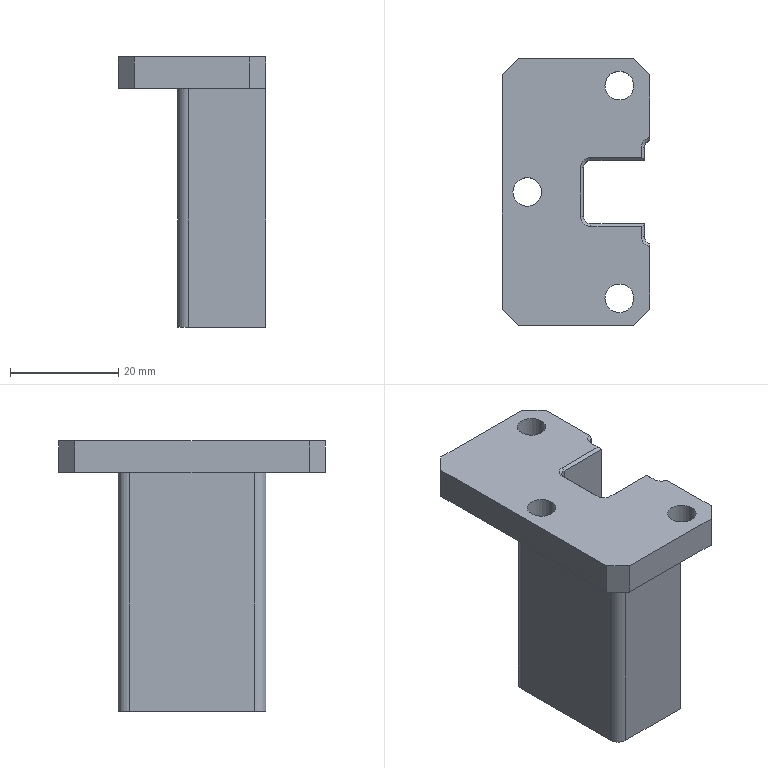Part | Creo | features CURVE 3, DATUM PLANE 3, CHAMFER 2, CUT 2, COORDINATE SYSTEM 1, PROTRUSION 1, ROUND 1 | 1 solid | 41 faces | volume 19348 mm3 | plane 25 | cylinder 12 | cone 4 | commonest cylinder face diameters 5.301 x6 2.75 x4 4 x2